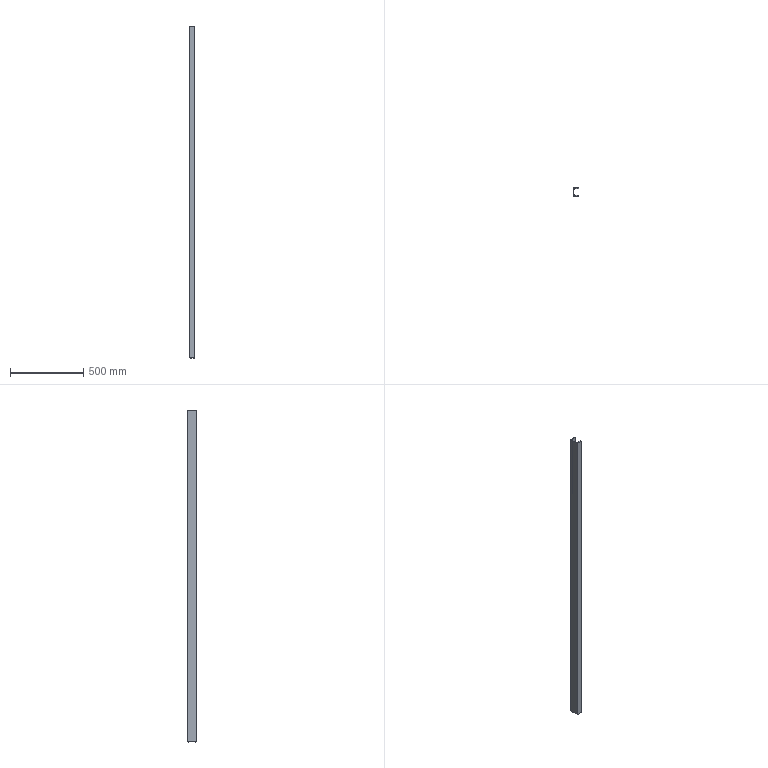Part | STEP file | 750038452 | 1 solid | 14 faces | box 40 x 63 x 2262 mm | volume 1910749 mm3 | plane 10 | cylinder 4 | commonest cylinder face diameters 7.6 x2 15 x2
STEP:
#1=CARTESIAN_POINT('',(0.,0.,1131.2));
#2=VERTEX_POINT('',#1);
#3=CARTESIAN_POINT('',(0.,0.,-1131.2));
#4=VERTEX_POINT('',#3);
#5=CARTESIAN_POINT('',(0.,0.,1131.2));
#6=DIRECTION('',(0.,0.,-1.));
#7=VECTOR('',#6,1000.);
#8=LINE('',#5,#7);
#9=EDGE_CURVE('',#2,#4,#8,.T.);
#10=ORIENTED_EDGE('',*,*,#9,.F.);
#11=CARTESIAN_POINT('',(0.,63.,1131.2));
#12=VERTEX_POINT('',#11);
#13=CARTESIAN_POINT('',(0.,63.,1131.2));
#14=DIRECTION('',(0.,-1.,0.));
#15=VECTOR('',#14,1000.);
#16=LINE('',#13,#15);
#17=EDGE_CURVE('',#12,#2,#16,.T.);
#18=ORIENTED_EDGE('',*,*,#17,.F.);
#19=CARTESIAN_POINT('',(0.,63.,-1131.2));
#20=VERTEX_POINT('',#19);
#21=CARTESIAN_POINT('',(0.,63.,1131.2));
#22=DIRECTION('',(0.,0.,1.));
#23=VECTOR('',#22,1000.);
#24=LINE('',#21,#23);
#25=EDGE_CURVE('',#20,#12,#24,.T.);
#26=ORIENTED_EDGE('',*,*,#25,.F.);
#27=CARTESIAN_POINT('',(0.,63.,-1131.2));
#28=DIRECTION('',(0.,1.,0.));
#29=VECTOR('',#28,1000.);
#30=LINE('',#27,#29);
#31=EDGE_CURVE('',#4,#20,#30,.T.);
#32=ORIENTED_EDGE('',*,*,#31,.F.);
#33=EDGE_LOOP('',(#10,#18,#26,#32));
#34=FACE_OUTER_BOUND('',#33,.T.);
#35=CARTESIAN_POINT('',(0.,63.,1131.2));
#36=DIRECTION('',(1.,0.,0.));
#37=DIRECTION('',(0.,0.,-1.));
#38=AXIS2_PLACEMENT_3D('',#35,#36,#37);
#39=PLANE('',#38);
#40=ADVANCED_FACE('',(#34),#39,.F.);
#41=CARTESIAN_POINT('',(40.,63.,-1131.2));
#42=VERTEX_POINT('',#41);
#43=CARTESIAN_POINT('',(36.2,63.,-1131.2));
#44=DIRECTION('',(-1.,0.,0.));
#45=VECTOR('',#44,1000.);
#46=LINE('',#43,#45);
#47=EDGE_CURVE('',#42,#20,#46,.T.);
#48=ORIENTED_EDGE('',*,*,#47,.F.);
#49=CARTESIAN_POINT('',(40.,60.699,-1131.2));
#50=VERTEX_POINT('',#49);
#51=CARTESIAN_POINT('',(40.,2.301,-1131.2));
#52=DIRECTION('',(0.,1.,0.));
#53=VECTOR('',#52,1000.);
#54=LINE('',#51,#53);
#55=EDGE_CURVE('',#50,#42,#54,.T.);
#56=ORIENTED_EDGE('',*,*,#55,.F.);
#57=CARTESIAN_POINT('',(36.578,56.918,-1131.2));
#58=VERTEX_POINT('',#57);
#59=CARTESIAN_POINT('',(36.2,60.699,-1131.2));
#60=DIRECTION('',(0.,0.,1.));
#61=DIRECTION('',(-1.,0.,0.));
#62=AXIS2_PLACEMENT_3D('',#59,#60,#61);
#63=CIRCLE('',#62,3.8);
#64=EDGE_CURVE('',#58,#50,#63,.T.);
#65=ORIENTED_EDGE('',*,*,#64,.F.);
#66=CARTESIAN_POINT('',(11.554,54.415,-1131.2));
#67=VERTEX_POINT('',#66);
#68=CARTESIAN_POINT('',(11.554,54.415,-1131.2));
#69=DIRECTION('',(0.995,0.0995,0.));
#70=VECTOR('',#69,1000.);
#71=LINE('',#68,#70);
#72=EDGE_CURVE('',#67,#58,#71,.T.);
#73=ORIENTED_EDGE('',*,*,#72,.F.);
#74=CARTESIAN_POINT('',(4.8,46.953,-1131.2));
#75=VERTEX_POINT('',#74);
#76=CARTESIAN_POINT('',(12.3,46.953,-1131.2));
#77=DIRECTION('',(0.,0.,-1.));
#78=DIRECTION('',(-1.,0.,0.));
#79=AXIS2_PLACEMENT_3D('',#76,#77,#78);
#80=CIRCLE('',#79,7.5);
#81=EDGE_CURVE('',#75,#67,#80,.T.);
#82=ORIENTED_EDGE('',*,*,#81,.F.);
#83=CARTESIAN_POINT('',(4.8,16.047,-1131.2));
#84=VERTEX_POINT('',#83);
#85=CARTESIAN_POINT('',(4.8,2.301,-1131.2));
#86=DIRECTION('',(0.,1.,0.));
#87=VECTOR('',#86,1000.);
#88=LINE('',#85,#87);
#89=EDGE_CURVE('',#84,#75,#88,.T.);
#90=ORIENTED_EDGE('',*,*,#89,.F.);
#91=CARTESIAN_POINT('',(11.554,8.585,-1131.2));
#92=VERTEX_POINT('',#91);
#93=CARTESIAN_POINT('',(12.3,16.047,-1131.2));
#94=DIRECTION('',(0.,0.,-1.));
#95=DIRECTION('',(-1.,0.,0.));
#96=AXIS2_PLACEMENT_3D('',#93,#94,#95);
#97=CIRCLE('',#96,7.5);
#98=EDGE_CURVE('',#92,#84,#97,.T.);
#99=ORIENTED_EDGE('',*,*,#98,.F.);
#100=CARTESIAN_POINT('',(36.578,6.082,-1131.2));
#101=VERTEX_POINT('',#100);
#102=CARTESIAN_POINT('',(36.578,6.082,-1131.2));
#103=DIRECTION('',(-0.995,0.0995,0.));
#104=VECTOR('',#103,1000.);
#105=LINE('',#102,#104);
#106=EDGE_CURVE('',#101,#92,#105,.T.);
#107=ORIENTED_EDGE('',*,*,#106,.F.);
#108=CARTESIAN_POINT('',(40.,2.301,-1131.2));
#109=VERTEX_POINT('',#108);
#110=CARTESIAN_POINT('',(36.2,2.301,-1131.2));
#111=DIRECTION('',(0.,0.,1.));
#112=DIRECTION('',(-1.,0.,0.));
#113=AXIS2_PLACEMENT_3D('',#110,#111,#112);
#114=CIRCLE('',#113,3.8);
#115=EDGE_CURVE('',#109,#101,#114,.T.);
#116=ORIENTED_EDGE('',*,*,#115,.F.);
#117=CARTESIAN_POINT('',(40.,0.,-1131.2));
#118=VERTEX_POINT('',#117);
#119=CARTESIAN_POINT('',(40.,2.301,-1131.2));
#120=DIRECTION('',(0.,1.,0.));
#121=VECTOR('',#120,1000.);
#122=LINE('',#119,#121);
#123=EDGE_CURVE('',#118,#109,#122,.T.);
#124=ORIENTED_EDGE('',*,*,#123,.F.);
#125=CARTESIAN_POINT('',(36.2,0.,-1131.2));
#126=DIRECTION('',(1.,0.,0.));
#127=VECTOR('',#126,1000.);
#128=LINE('',#125,#127);
#129=EDGE_CURVE('',#4,#118,#128,.T.);
#130=ORIENTED_EDGE('',*,*,#129,.F.);
#131=ORIENTED_EDGE('',*,*,#31,.T.);
#132=EDGE_LOOP('',(#48,#56,#65,#73,#82,#90,#99,#107,#116,#124,#130,#131));
#133=FACE_OUTER_BOUND('',#132,.T.);
#134=CARTESIAN_POINT('',(36.2,2.301,-1131.2));
#135=DIRECTION('',(0.,0.,1.));
#136=DIRECTION('',(1.,0.,0.));
#137=AXIS2_PLACEMENT_3D('',#134,#135,#136);
#138=PLANE('',#137);
#139=ADVANCED_FACE('',(#133),#138,.F.);
#140=CARTESIAN_POINT('',(40.,0.,1131.2));
#141=VERTEX_POINT('',#140);
#142=CARTESIAN_POINT('',(40.,0.,1131.2));
#143=DIRECTION('',(0.,0.,-1.));
#144=VECTOR('',#143,1000.);
#145=LINE('',#142,#144);
#146=EDGE_CURVE('',#141,#118,#145,.T.);
#147=ORIENTED_EDGE('',*,*,#146,.F.);
#148=CARTESIAN_POINT('',(0.,0.,1131.2));
#149=DIRECTION('',(1.,0.,0.));
#150=VECTOR('',#149,1000.);
#151=LINE('',#148,#150);
#152=EDGE_CURVE('',#2,#141,#151,.T.);
#153=ORIENTED_EDGE('',*,*,#152,.F.);
#154=ORIENTED_EDGE('',*,*,#9,.T.);
#155=ORIENTED_EDGE('',*,*,#129,.T.);
#156=EDGE_LOOP('',(#147,#153,#154,#155));
#157=FACE_OUTER_BOUND('',#156,.T.);
#158=CARTESIAN_POINT('',(0.,0.,1131.2));
#159=DIRECTION('',(0.,1.,0.));
#160=DIRECTION('',(0.,0.,1.));
#161=AXIS2_PLACEMENT_3D('',#158,#159,#160);
#162=PLANE('',#161);
#163=ADVANCED_FACE('',(#157),#162,.F.);
#164=CARTESIAN_POINT('',(40.,60.699,1131.2));
#165=VERTEX_POINT('',#164);
#166=CARTESIAN_POINT('',(40.,63.,1131.2));
#167=VERTEX_POINT('',#166);
#168=CARTESIAN_POINT('',(40.,2.301,1131.2));
#169=DIRECTION('',(0.,1.,0.));
#170=VECTOR('',#169,1000.);
#171=LINE('',#168,#170);
#172=EDGE_CURVE('',#165,#167,#171,.T.);
#173=ORIENTED_EDGE('',*,*,#172,.T.);
#174=CARTESIAN_POINT('',(36.2,63.,1131.2));
#175=DIRECTION('',(-1.,0.,0.));
#176=VECTOR('',#175,1000.);
#177=LINE('',#174,#176);
#178=EDGE_CURVE('',#167,#12,#177,.T.);
#179=ORIENTED_EDGE('',*,*,#178,.T.);
#180=ORIENTED_EDGE('',*,*,#17,.T.);
#181=ORIENTED_EDGE('',*,*,#152,.T.);
#182=CARTESIAN_POINT('',(40.,2.301,1131.2));
#183=VERTEX_POINT('',#182);
#184=CARTESIAN_POINT('',(40.,2.301,1131.2));
#185=DIRECTION('',(0.,1.,0.));
#186=VECTOR('',#185,1000.);
#187=LINE('',#184,#186);
#188=EDGE_CURVE('',#141,#183,#187,.T.);
#189=ORIENTED_EDGE('',*,*,#188,.T.);
#190=CARTESIAN_POINT('',(36.578,6.082,1131.2));
#191=VERTEX_POINT('',#190);
#192=CARTESIAN_POINT('',(36.2,2.301,1131.2));
#193=DIRECTION('',(0.,0.,1.));
#194=DIRECTION('',(-1.,0.,0.));
#195=AXIS2_PLACEMENT_3D('',#192,#193,#194);
#196=CIRCLE('',#195,3.8);
#197=EDGE_CURVE('',#183,#191,#196,.T.);
#198=ORIENTED_EDGE('',*,*,#197,.T.);
#199=CARTESIAN_POINT('',(11.554,8.585,1131.2));
#200=VERTEX_POINT('',#199);
#201=CARTESIAN_POINT('',(36.578,6.082,1131.2));
#202=DIRECTION('',(-0.995,0.0995,0.));
#203=VECTOR('',#202,1000.);
#204=LINE('',#201,#203);
#205=EDGE_CURVE('',#191,#200,#204,.T.);
#206=ORIENTED_EDGE('',*,*,#205,.T.);
#207=CARTESIAN_POINT('',(4.8,16.047,1131.2));
#208=VERTEX_POINT('',#207);
#209=CARTESIAN_POINT('',(12.3,16.047,1131.2));
#210=DIRECTION('',(0.,0.,-1.));
#211=DIRECTION('',(-1.,0.,0.));
#212=AXIS2_PLACEMENT_3D('',#209,#210,#211);
#213=CIRCLE('',#212,7.5);
#214=EDGE_CURVE('',#200,#208,#213,.T.);
#215=ORIENTED_EDGE('',*,*,#214,.T.);
#216=CARTESIAN_POINT('',(4.8,46.953,1131.2));
#217=VERTEX_POINT('',#216);
#218=CARTESIAN_POINT('',(4.8,2.301,1131.2));
#219=DIRECTION('',(0.,1.,0.));
#220=VECTOR('',#219,1000.);
#221=LINE('',#218,#220);
#222=EDGE_CURVE('',#208,#217,#221,.T.);
#223=ORIENTED_EDGE('',*,*,#222,.T.);
#224=CARTESIAN_POINT('',(11.554,54.415,1131.2));
#225=VERTEX_POINT('',#224);
#226=CARTESIAN_POINT('',(12.3,46.953,1131.2));
#227=DIRECTION('',(0.,0.,-1.));
#228=DIRECTION('',(-1.,0.,0.));
#229=AXIS2_PLACEMENT_3D('',#226,#227,#228);
#230=CIRCLE('',#229,7.5);
#231=EDGE_CURVE('',#217,#225,#230,.T.);
#232=ORIENTED_EDGE('',*,*,#231,.T.);
#233=CARTESIAN_POINT('',(36.578,56.918,1131.2));
#234=VERTEX_POINT('',#233);
#235=CARTESIAN_POINT('',(11.554,54.415,1131.2));
#236=DIRECTION('',(0.995,0.0995,0.));
#237=VECTOR('',#236,1000.);
#238=LINE('',#235,#237);
#239=EDGE_CURVE('',#225,#234,#238,.T.);
#240=ORIENTED_EDGE('',*,*,#239,.T.);
#241=CARTESIAN_POINT('',(36.2,60.699,1131.2));
#242=DIRECTION('',(0.,0.,1.));
#243=DIRECTION('',(-1.,0.,0.));
#244=AXIS2_PLACEMENT_3D('',#241,#242,#243);
#245=CIRCLE('',#244,3.8);
#246=EDGE_CURVE('',#234,#165,#245,.T.);
#247=ORIENTED_EDGE('',*,*,#246,.T.);
#248=EDGE_LOOP('',(#173,#179,#180,#181,#189,#198,#206,#215,#223,#232,#240,#247));
#249=FACE_OUTER_BOUND('',#248,.T.);
#250=CARTESIAN_POINT('',(36.2,2.301,1131.2));
#251=DIRECTION('',(0.,0.,1.));
#252=DIRECTION('',(1.,0.,0.));
#253=AXIS2_PLACEMENT_3D('',#250,#251,#252);
#254=PLANE('',#253);
#255=ADVANCED_FACE('',(#249),#254,.T.);
#256=ORIENTED_EDGE('',*,*,#25,.T.);
#257=ORIENTED_EDGE('',*,*,#178,.F.);
#258=CARTESIAN_POINT('',(40.,63.,1131.2));
#259=DIRECTION('',(0.,0.,1.));
#260=VECTOR('',#259,1000.);
#261=LINE('',#258,#260);
#262=EDGE_CURVE('',#42,#167,#261,.T.);
#263=ORIENTED_EDGE('',*,*,#262,.F.);
#264=ORIENTED_EDGE('',*,*,#47,.T.);
#265=EDGE_LOOP('',(#256,#257,#263,#264));
#266=FACE_OUTER_BOUND('',#265,.T.);
#267=CARTESIAN_POINT('',(40.,63.,1131.2));
#268=DIRECTION('',(0.,-1.,0.));
#269=DIRECTION('',(0.,0.,-1.));
#270=AXIS2_PLACEMENT_3D('',#267,#268,#269);
#271=PLANE('',#270);
#272=ADVANCED_FACE('',(#266),#271,.F.);
#273=ORIENTED_EDGE('',*,*,#262,.T.);
#274=ORIENTED_EDGE('',*,*,#172,.F.);
#275=CARTESIAN_POINT('',(40.,60.699,1131.2));
#276=DIRECTION('',(0.,0.,1.));
#277=VECTOR('',#276,1000.);
#278=LINE('',#275,#277);
#279=EDGE_CURVE('',#50,#165,#278,.T.);
#280=ORIENTED_EDGE('',*,*,#279,.F.);
#281=ORIENTED_EDGE('',*,*,#55,.T.);
#282=EDGE_LOOP('',(#273,#274,#280,#281));
#283=FACE_OUTER_BOUND('',#282,.T.);
#284=CARTESIAN_POINT('',(40.,60.699,1131.2));
#285=DIRECTION('',(-1.,0.,0.));
#286=DIRECTION('',(0.,-1.,0.));
#287=AXIS2_PLACEMENT_3D('',#284,#285,#286);
#288=PLANE('',#287);
#289=ADVANCED_FACE('',(#283),#288,.F.);
#290=ORIENTED_EDGE('',*,*,#246,.F.);
#291=CARTESIAN_POINT('',(36.578,56.918,1131.2));
#292=DIRECTION('',(0.,0.,-1.));
#293=VECTOR('',#292,1000.);
#294=LINE('',#291,#293);
#295=EDGE_CURVE('',#234,#58,#294,.T.);
#296=ORIENTED_EDGE('',*,*,#295,.T.);
#297=ORIENTED_EDGE('',*,*,#64,.T.);
#298=ORIENTED_EDGE('',*,*,#279,.T.);
#299=EDGE_LOOP('',(#290,#296,#297,#298));
#300=FACE_OUTER_BOUND('',#299,.T.);
#301=CARTESIAN_POINT('',(36.2,60.699,1131.2));
#302=DIRECTION('',(0.,0.,-1.));
#303=DIRECTION('',(-1.,0.,0.));
#304=AXIS2_PLACEMENT_3D('',#301,#302,#303);
#305=CYLINDRICAL_SURFACE('',#304,3.8);
#306=ADVANCED_FACE('',(#300),#305,.T.);
#307=ORIENTED_EDGE('',*,*,#295,.F.);
#308=ORIENTED_EDGE('',*,*,#239,.F.);
#309=CARTESIAN_POINT('',(11.554,54.415,1131.2));
#310=DIRECTION('',(0.,0.,1.));
#311=VECTOR('',#310,1000.);
#312=LINE('',#309,#311);
#313=EDGE_CURVE('',#67,#225,#312,.T.);
#314=ORIENTED_EDGE('',*,*,#313,.F.);
#315=ORIENTED_EDGE('',*,*,#72,.T.);
#316=EDGE_LOOP('',(#307,#308,#314,#315));
#317=FACE_OUTER_BOUND('',#316,.T.);
#318=CARTESIAN_POINT('',(11.554,54.415,1131.2));
#319=DIRECTION('',(-0.0995,0.995,0.));
#320=DIRECTION('',(-0.995,-0.0995,0.));
#321=AXIS2_PLACEMENT_3D('',#318,#319,#320);
#322=PLANE('',#321);
#323=ADVANCED_FACE('',(#317),#322,.F.);
#324=ORIENTED_EDGE('',*,*,#313,.T.);
#325=ORIENTED_EDGE('',*,*,#231,.F.);
#326=CARTESIAN_POINT('',(4.8,46.953,1131.2));
#327=DIRECTION('',(0.,0.,1.));
#328=VECTOR('',#327,1000.);
#329=LINE('',#326,#328);
#330=EDGE_CURVE('',#75,#217,#329,.T.);
#331=ORIENTED_EDGE('',*,*,#330,.F.);
#332=ORIENTED_EDGE('',*,*,#81,.T.);
#333=EDGE_LOOP('',(#324,#325,#331,#332));
#334=FACE_OUTER_BOUND('',#333,.T.);
#335=CARTESIAN_POINT('',(12.3,46.953,1131.2));
#336=DIRECTION('',(0.,0.,-1.));
#337=DIRECTION('',(-1.,0.,0.));
#338=AXIS2_PLACEMENT_3D('',#335,#336,#337);
#339=CYLINDRICAL_SURFACE('',#338,7.5);
#340=ADVANCED_FACE('',(#334),#339,.F.);
#341=ORIENTED_EDGE('',*,*,#330,.T.);
#342=ORIENTED_EDGE('',*,*,#222,.F.);
#343=CARTESIAN_POINT('',(4.8,16.047,1131.2));
#344=DIRECTION('',(0.,0.,1.));
#345=VECTOR('',#344,1000.);
#346=LINE('',#343,#345);
#347=EDGE_CURVE('',#84,#208,#346,.T.);
#348=ORIENTED_EDGE('',*,*,#347,.F.);
#349=ORIENTED_EDGE('',*,*,#89,.T.);
#350=EDGE_LOOP('',(#341,#342,#348,#349));
#351=FACE_OUTER_BOUND('',#350,.T.);
#352=CARTESIAN_POINT('',(4.8,16.047,1131.2));
#353=DIRECTION('',(-1.,0.,0.));
#354=DIRECTION('',(0.,-1.,0.));
#355=AXIS2_PLACEMENT_3D('',#352,#353,#354);
#356=PLANE('',#355);
#357=ADVANCED_FACE('',(#351),#356,.F.);
#358=ORIENTED_EDGE('',*,*,#347,.T.);
#359=ORIENTED_EDGE('',*,*,#214,.F.);
#360=CARTESIAN_POINT('',(11.554,8.585,1131.2));
#361=DIRECTION('',(0.,0.,1.));
#362=VECTOR('',#361,1000.);
#363=LINE('',#360,#362);
#364=EDGE_CURVE('',#92,#200,#363,.T.);
#365=ORIENTED_EDGE('',*,*,#364,.F.);
#366=ORIENTED_EDGE('',*,*,#98,.T.);
#367=EDGE_LOOP('',(#358,#359,#365,#366));
#368=FACE_OUTER_BOUND('',#367,.T.);
#369=CARTESIAN_POINT('',(12.3,16.047,1131.2));
#370=DIRECTION('',(0.,0.,-1.));
#371=DIRECTION('',(-1.,0.,0.));
#372=AXIS2_PLACEMENT_3D('',#369,#370,#371);
#373=CYLINDRICAL_SURFACE('',#372,7.5);
#374=ADVANCED_FACE('',(#368),#373,.F.);
#375=ORIENTED_EDGE('',*,*,#364,.T.);
#376=ORIENTED_EDGE('',*,*,#205,.F.);
#377=CARTESIAN_POINT('',(36.578,6.082,1131.2));
#378=DIRECTION('',(0.,0.,1.));
#379=VECTOR('',#378,1000.);
#380=LINE('',#377,#379);
#381=EDGE_CURVE('',#101,#191,#380,.T.);
#382=ORIENTED_EDGE('',*,*,#381,.F.);
#383=ORIENTED_EDGE('',*,*,#106,.T.);
#384=EDGE_LOOP('',(#375,#376,#382,#383));
#385=FACE_OUTER_BOUND('',#384,.T.);
#386=CARTESIAN_POINT('',(36.578,6.082,1131.2));
#387=DIRECTION('',(-0.0995,-0.995,0.));
#388=DIRECTION('',(0.995,-0.0995,0.));
#389=AXIS2_PLACEMENT_3D('',#386,#387,#388);
#390=PLANE('',#389);
#391=ADVANCED_FACE('',(#385),#390,.F.);
#392=ORIENTED_EDGE('',*,*,#197,.F.);
#393=CARTESIAN_POINT('',(40.,2.301,1131.2));
#394=DIRECTION('',(0.,0.,-1.));
#395=VECTOR('',#394,1000.);
#396=LINE('',#393,#395);
#397=EDGE_CURVE('',#183,#109,#396,.T.);
#398=ORIENTED_EDGE('',*,*,#397,.T.);
#399=ORIENTED_EDGE('',*,*,#115,.T.);
#400=ORIENTED_EDGE('',*,*,#381,.T.);
#401=EDGE_LOOP('',(#392,#398,#399,#400));
#402=FACE_OUTER_BOUND('',#401,.T.);
#403=CARTESIAN_POINT('',(36.2,2.301,1131.2));
#404=DIRECTION('',(0.,0.,-1.));
#405=DIRECTION('',(-1.,0.,0.));
#406=AXIS2_PLACEMENT_3D('',#403,#404,#405);
#407=CYLINDRICAL_SURFACE('',#406,3.8);
#408=ADVANCED_FACE('',(#402),#407,.T.);
#409=ORIENTED_EDGE('',*,*,#397,.F.);
#410=ORIENTED_EDGE('',*,*,#188,.F.);
#411=ORIENTED_EDGE('',*,*,#146,.T.);
#412=ORIENTED_EDGE('',*,*,#123,.T.);
#413=EDGE_LOOP('',(#409,#410,#411,#412));
#414=FACE_OUTER_BOUND('',#413,.T.);
#415=CARTESIAN_POINT('',(40.,0.,1131.2));
#416=DIRECTION('',(-1.,0.,0.));
#417=DIRECTION('',(0.,0.,1.));
#418=AXIS2_PLACEMENT_3D('',#415,#416,#417);
#419=PLANE('',#418);
#420=ADVANCED_FACE('',(#414),#419,.F.);
#421=CLOSED_SHELL('',(#40,#139,#163,#255,#272,#289,#306,#323,#340,#357,#374,#391,#408,#420));
#422=MANIFOLD_SOLID_BREP('',#421);
#423=CARTESIAN_POINT('',(0.,0.,0.));
#424=DIRECTION('',(0.,0.,1.));
#425=DIRECTION('',(1.,0.,0.));
#426=AXIS2_PLACEMENT_3D('',#423,#424,#425);
#427=(LENGTH_UNIT()NAMED_UNIT(*)SI_UNIT(.MILLI.,.METRE.));
#428=UNCERTAINTY_MEASURE_WITH_UNIT(LENGTH_MEASURE(0.00001),#427,'','');
#429=(NAMED_UNIT(*)PLANE_ANGLE_UNIT()SI_UNIT($,.RADIAN.));
#430=(NAMED_UNIT(*)SI_UNIT($,.STERADIAN.)SOLID_ANGLE_UNIT());
#431=(GEOMETRIC_REPRESENTATION_CONTEXT(3)GLOBAL_UNCERTAINTY_ASSIGNED_CONTEXT((#428))GLOBAL_UNIT_ASSIGNED_CONTEXT((#427,#429,#430))REPRESENTATION_CONTEXT('',''));
#432=ADVANCED_BREP_SHAPE_REPRESENTATION('',(#422,#426),#431);